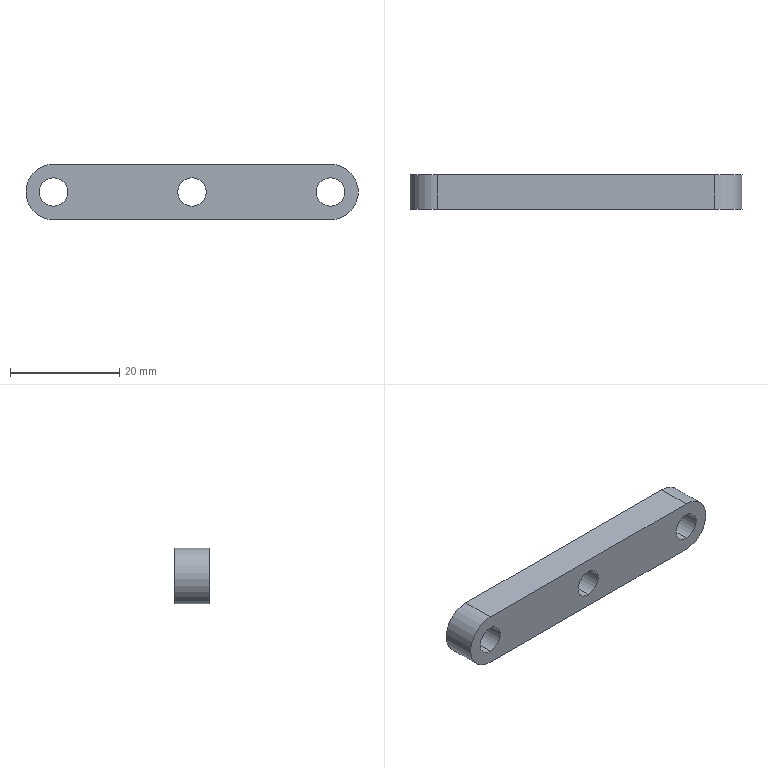Part | SolidWorks | features ICE 2, Extrusion 1 | 1 solid | 12 faces | box 60.96 x 6.35 x 10.16 mm | volume 3387 mm3 | cylinder 8 | plane 4 | commonest cylinder face diameters 5.207 x6 10.16 x2
STEP:
#1=CARTESIAN_POINT('',(25.4,0.,-2.604));
#2=VERTEX_POINT('',#1);
#3=CARTESIAN_POINT('',(25.4,0.,2.604));
#4=VERTEX_POINT('',#3);
#5=CARTESIAN_POINT('',(25.4,0.,0.));
#6=DIRECTION('',(0.,1.,0.));
#7=DIRECTION('',(0.,0.,1.));
#8=AXIS2_PLACEMENT_3D('',#5,#6,#7);
#9=CIRCLE('',#8,2.604);
#10=EDGE_CURVE('',#2,#4,#9,.T.);
#11=ORIENTED_EDGE('',*,*,#10,.F.);
#12=CARTESIAN_POINT('',(25.4,6.35,-2.604));
#13=VERTEX_POINT('',#12);
#14=CARTESIAN_POINT('',(25.4,0.,-2.604));
#15=DIRECTION('',(0.,1.,0.));
#16=VECTOR('',#15,1000.);
#17=LINE('',#14,#16);
#18=EDGE_CURVE('',#2,#13,#17,.T.);
#19=ORIENTED_EDGE('',*,*,#18,.T.);
#20=CARTESIAN_POINT('',(25.4,6.35,2.604));
#21=VERTEX_POINT('',#20);
#22=CARTESIAN_POINT('',(25.4,6.35,0.));
#23=DIRECTION('',(0.,1.,0.));
#24=DIRECTION('',(0.,0.,1.));
#25=AXIS2_PLACEMENT_3D('',#22,#23,#24);
#26=CIRCLE('',#25,2.604);
#27=EDGE_CURVE('',#13,#21,#26,.T.);
#28=ORIENTED_EDGE('',*,*,#27,.T.);
#29=CARTESIAN_POINT('',(25.4,0.,2.604));
#30=DIRECTION('',(0.,1.,0.));
#31=VECTOR('',#30,1000.);
#32=LINE('',#29,#31);
#33=EDGE_CURVE('',#4,#21,#32,.T.);
#34=ORIENTED_EDGE('',*,*,#33,.F.);
#35=EDGE_LOOP('',(#11,#19,#28,#34));
#36=FACE_OUTER_BOUND('',#35,.T.);
#37=CARTESIAN_POINT('',(25.4,0.,0.));
#38=DIRECTION('',(0.,1.,0.));
#39=DIRECTION('',(0.,0.,1.));
#40=AXIS2_PLACEMENT_3D('',#37,#38,#39);
#41=CYLINDRICAL_SURFACE('',#40,2.604);
#42=ADVANCED_FACE('',(#36),#41,.F.);
#43=CARTESIAN_POINT('',(50.8,0.,-2.604));
#44=VERTEX_POINT('',#43);
#45=CARTESIAN_POINT('',(50.8,0.,2.604));
#46=VERTEX_POINT('',#45);
#47=CARTESIAN_POINT('',(50.8,0.,0.));
#48=DIRECTION('',(0.,1.,0.));
#49=DIRECTION('',(0.,0.,-1.));
#50=AXIS2_PLACEMENT_3D('',#47,#48,#49);
#51=CIRCLE('',#50,2.604);
#52=EDGE_CURVE('',#44,#46,#51,.T.);
#53=ORIENTED_EDGE('',*,*,#52,.F.);
#54=CARTESIAN_POINT('',(50.8,6.35,-2.604));
#55=VERTEX_POINT('',#54);
#56=CARTESIAN_POINT('',(50.8,-8.202,-2.604));
#57=DIRECTION('',(0.,1.,0.));
#58=VECTOR('',#57,1000.);
#59=LINE('',#56,#58);
#60=EDGE_CURVE('',#44,#55,#59,.T.);
#61=ORIENTED_EDGE('',*,*,#60,.T.);
#62=CARTESIAN_POINT('',(50.8,6.35,2.604));
#63=VERTEX_POINT('',#62);
#64=CARTESIAN_POINT('',(50.8,6.35,0.));
#65=DIRECTION('',(0.,1.,0.));
#66=DIRECTION('',(0.,0.,1.));
#67=AXIS2_PLACEMENT_3D('',#64,#65,#66);
#68=CIRCLE('',#67,2.604);
#69=EDGE_CURVE('',#55,#63,#68,.T.);
#70=ORIENTED_EDGE('',*,*,#69,.T.);
#71=CARTESIAN_POINT('',(50.8,-8.202,2.604));
#72=DIRECTION('',(0.,1.,0.));
#73=VECTOR('',#72,1000.);
#74=LINE('',#71,#73);
#75=EDGE_CURVE('',#46,#63,#74,.T.);
#76=ORIENTED_EDGE('',*,*,#75,.F.);
#77=EDGE_LOOP('',(#53,#61,#70,#76));
#78=FACE_OUTER_BOUND('',#77,.T.);
#79=CARTESIAN_POINT('',(50.8,-8.202,0.));
#80=DIRECTION('',(0.,1.,0.));
#81=DIRECTION('',(0.,0.,1.));
#82=AXIS2_PLACEMENT_3D('',#79,#80,#81);
#83=CYLINDRICAL_SURFACE('',#82,2.604);
#84=ADVANCED_FACE('',(#78),#83,.F.);
#85=CARTESIAN_POINT('',(0.,0.,-2.603));
#86=VERTEX_POINT('',#85);
#87=CARTESIAN_POINT('',(0.,0.,2.603));
#88=VERTEX_POINT('',#87);
#89=CARTESIAN_POINT('',(0.,0.,0.));
#90=DIRECTION('',(0.,1.,0.));
#91=DIRECTION('',(0.,0.,-1.));
#92=AXIS2_PLACEMENT_3D('',#89,#90,#91);
#93=CIRCLE('',#92,2.603);
#94=EDGE_CURVE('',#86,#88,#93,.T.);
#95=ORIENTED_EDGE('',*,*,#94,.F.);
#96=CARTESIAN_POINT('',(0.,6.35,-2.603));
#97=VERTEX_POINT('',#96);
#98=CARTESIAN_POINT('',(0.,-8.202,-2.603));
#99=DIRECTION('',(0.,1.,0.));
#100=VECTOR('',#99,1000.);
#101=LINE('',#98,#100);
#102=EDGE_CURVE('',#86,#97,#101,.T.);
#103=ORIENTED_EDGE('',*,*,#102,.T.);
#104=CARTESIAN_POINT('',(0.,6.35,2.603));
#105=VERTEX_POINT('',#104);
#106=CARTESIAN_POINT('',(0.,6.35,0.));
#107=DIRECTION('',(0.,1.,0.));
#108=DIRECTION('',(0.,0.,1.));
#109=AXIS2_PLACEMENT_3D('',#106,#107,#108);
#110=CIRCLE('',#109,2.603);
#111=EDGE_CURVE('',#97,#105,#110,.T.);
#112=ORIENTED_EDGE('',*,*,#111,.T.);
#113=CARTESIAN_POINT('',(0.,-8.202,2.603));
#114=DIRECTION('',(0.,1.,0.));
#115=VECTOR('',#114,1000.);
#116=LINE('',#113,#115);
#117=EDGE_CURVE('',#88,#105,#116,.T.);
#118=ORIENTED_EDGE('',*,*,#117,.F.);
#119=EDGE_LOOP('',(#95,#103,#112,#118));
#120=FACE_OUTER_BOUND('',#119,.T.);
#121=CARTESIAN_POINT('',(0.,-8.202,0.));
#122=DIRECTION('',(0.,1.,0.));
#123=DIRECTION('',(0.,0.,1.));
#124=AXIS2_PLACEMENT_3D('',#121,#122,#123);
#125=CYLINDRICAL_SURFACE('',#124,2.603);
#126=ADVANCED_FACE('',(#120),#125,.F.);
#127=CARTESIAN_POINT('',(25.4,6.35,0.));
#128=DIRECTION('',(0.,1.,0.));
#129=DIRECTION('',(0.,0.,1.));
#130=AXIS2_PLACEMENT_3D('',#127,#128,#129);
#131=CIRCLE('',#130,2.604);
#132=EDGE_CURVE('',#21,#13,#131,.T.);
#133=ORIENTED_EDGE('',*,*,#132,.F.);
#134=ORIENTED_EDGE('',*,*,#27,.F.);
#135=EDGE_LOOP('',(#133,#134));
#136=FACE_BOUND('',#135,.T.);
#137=CARTESIAN_POINT('',(0.,6.35,-5.08));
#138=VERTEX_POINT('',#137);
#139=CARTESIAN_POINT('',(0.,6.35,5.08));
#140=VERTEX_POINT('',#139);
#141=CARTESIAN_POINT('',(0.,6.35,0.));
#142=DIRECTION('',(0.,1.,0.));
#143=DIRECTION('',(0.,0.,-1.));
#144=AXIS2_PLACEMENT_3D('',#141,#142,#143);
#145=CIRCLE('',#144,5.08);
#146=EDGE_CURVE('',#138,#140,#145,.T.);
#147=ORIENTED_EDGE('',*,*,#146,.T.);
#148=CARTESIAN_POINT('',(50.8,6.35,5.08));
#149=VERTEX_POINT('',#148);
#150=CARTESIAN_POINT('',(0.,6.35,5.08));
#151=DIRECTION('',(1.,0.,0.));
#152=VECTOR('',#151,1000.);
#153=LINE('',#150,#152);
#154=EDGE_CURVE('',#140,#149,#153,.T.);
#155=ORIENTED_EDGE('',*,*,#154,.T.);
#156=CARTESIAN_POINT('',(50.8,6.35,-5.08));
#157=VERTEX_POINT('',#156);
#158=CARTESIAN_POINT('',(50.8,6.35,0.));
#159=DIRECTION('',(0.,1.,0.));
#160=DIRECTION('',(0.,0.,-1.));
#161=AXIS2_PLACEMENT_3D('',#158,#159,#160);
#162=CIRCLE('',#161,5.08);
#163=EDGE_CURVE('',#149,#157,#162,.T.);
#164=ORIENTED_EDGE('',*,*,#163,.T.);
#165=CARTESIAN_POINT('',(0.,6.35,-5.08));
#166=DIRECTION('',(-1.,0.,0.));
#167=VECTOR('',#166,1000.);
#168=LINE('',#165,#167);
#169=EDGE_CURVE('',#157,#138,#168,.T.);
#170=ORIENTED_EDGE('',*,*,#169,.T.);
#171=EDGE_LOOP('',(#147,#155,#164,#170));
#172=FACE_OUTER_BOUND('',#171,.T.);
#173=CARTESIAN_POINT('',(0.,6.35,0.));
#174=DIRECTION('',(0.,1.,0.));
#175=DIRECTION('',(0.,0.,1.));
#176=AXIS2_PLACEMENT_3D('',#173,#174,#175);
#177=CIRCLE('',#176,2.603);
#178=EDGE_CURVE('',#105,#97,#177,.T.);
#179=ORIENTED_EDGE('',*,*,#178,.F.);
#180=ORIENTED_EDGE('',*,*,#111,.F.);
#181=EDGE_LOOP('',(#179,#180));
#182=FACE_BOUND('',#181,.T.);
#183=CARTESIAN_POINT('',(50.8,6.35,0.));
#184=DIRECTION('',(0.,1.,0.));
#185=DIRECTION('',(0.,0.,1.));
#186=AXIS2_PLACEMENT_3D('',#183,#184,#185);
#187=CIRCLE('',#186,2.604);
#188=EDGE_CURVE('',#63,#55,#187,.T.);
#189=ORIENTED_EDGE('',*,*,#188,.F.);
#190=ORIENTED_EDGE('',*,*,#69,.F.);
#191=EDGE_LOOP('',(#189,#190));
#192=FACE_BOUND('',#191,.T.);
#193=CARTESIAN_POINT('',(0.,6.35,0.));
#194=DIRECTION('',(0.,-1.,0.));
#195=DIRECTION('',(0.,0.,-1.));
#196=AXIS2_PLACEMENT_3D('',#193,#194,#195);
#197=PLANE('',#196);
#198=ADVANCED_FACE('',(#136,#172,#182,#192),#197,.F.);
#199=CARTESIAN_POINT('',(25.4,0.,0.));
#200=DIRECTION('',(0.,1.,0.));
#201=DIRECTION('',(0.,0.,1.));
#202=AXIS2_PLACEMENT_3D('',#199,#200,#201);
#203=CIRCLE('',#202,2.604);
#204=EDGE_CURVE('',#4,#2,#203,.T.);
#205=ORIENTED_EDGE('',*,*,#204,.T.);
#206=ORIENTED_EDGE('',*,*,#10,.T.);
#207=EDGE_LOOP('',(#205,#206));
#208=FACE_BOUND('',#207,.T.);
#209=CARTESIAN_POINT('',(0.,0.,-5.08));
#210=VERTEX_POINT('',#209);
#211=CARTESIAN_POINT('',(0.,0.,5.08));
#212=VERTEX_POINT('',#211);
#213=CARTESIAN_POINT('',(0.,0.,0.));
#214=DIRECTION('',(0.,1.,0.));
#215=DIRECTION('',(0.,0.,-1.));
#216=AXIS2_PLACEMENT_3D('',#213,#214,#215);
#217=CIRCLE('',#216,5.08);
#218=EDGE_CURVE('',#210,#212,#217,.T.);
#219=ORIENTED_EDGE('',*,*,#218,.F.);
#220=CARTESIAN_POINT('',(50.8,0.,-5.08));
#221=VERTEX_POINT('',#220);
#222=CARTESIAN_POINT('',(0.,0.,-5.08));
#223=DIRECTION('',(-1.,0.,0.));
#224=VECTOR('',#223,1000.);
#225=LINE('',#222,#224);
#226=EDGE_CURVE('',#221,#210,#225,.T.);
#227=ORIENTED_EDGE('',*,*,#226,.F.);
#228=CARTESIAN_POINT('',(50.8,0.,5.08));
#229=VERTEX_POINT('',#228);
#230=CARTESIAN_POINT('',(50.8,0.,0.));
#231=DIRECTION('',(0.,1.,0.));
#232=DIRECTION('',(0.,0.,-1.));
#233=AXIS2_PLACEMENT_3D('',#230,#231,#232);
#234=CIRCLE('',#233,5.08);
#235=EDGE_CURVE('',#229,#221,#234,.T.);
#236=ORIENTED_EDGE('',*,*,#235,.F.);
#237=CARTESIAN_POINT('',(0.,0.,5.08));
#238=DIRECTION('',(1.,0.,0.));
#239=VECTOR('',#238,1000.);
#240=LINE('',#237,#239);
#241=EDGE_CURVE('',#212,#229,#240,.T.);
#242=ORIENTED_EDGE('',*,*,#241,.F.);
#243=EDGE_LOOP('',(#219,#227,#236,#242));
#244=FACE_OUTER_BOUND('',#243,.T.);
#245=CARTESIAN_POINT('',(0.,0.,0.));
#246=DIRECTION('',(0.,1.,0.));
#247=DIRECTION('',(0.,0.,-1.));
#248=AXIS2_PLACEMENT_3D('',#245,#246,#247);
#249=CIRCLE('',#248,2.603);
#250=EDGE_CURVE('',#88,#86,#249,.T.);
#251=ORIENTED_EDGE('',*,*,#250,.T.);
#252=ORIENTED_EDGE('',*,*,#94,.T.);
#253=EDGE_LOOP('',(#251,#252));
#254=FACE_BOUND('',#253,.T.);
#255=CARTESIAN_POINT('',(50.8,0.,0.));
#256=DIRECTION('',(0.,1.,0.));
#257=DIRECTION('',(0.,0.,-1.));
#258=AXIS2_PLACEMENT_3D('',#255,#256,#257);
#259=CIRCLE('',#258,2.604);
#260=EDGE_CURVE('',#46,#44,#259,.T.);
#261=ORIENTED_EDGE('',*,*,#260,.T.);
#262=ORIENTED_EDGE('',*,*,#52,.T.);
#263=EDGE_LOOP('',(#261,#262));
#264=FACE_BOUND('',#263,.T.);
#265=CARTESIAN_POINT('',(0.,0.,0.));
#266=DIRECTION('',(0.,-1.,0.));
#267=DIRECTION('',(0.,0.,-1.));
#268=AXIS2_PLACEMENT_3D('',#265,#266,#267);
#269=PLANE('',#268);
#270=ADVANCED_FACE('',(#208,#244,#254,#264),#269,.T.);
#271=ORIENTED_EDGE('',*,*,#218,.T.);
#272=CARTESIAN_POINT('',(0.,6.35,5.08));
#273=DIRECTION('',(0.,-1.,0.));
#274=VECTOR('',#273,1000.);
#275=LINE('',#272,#274);
#276=EDGE_CURVE('',#140,#212,#275,.T.);
#277=ORIENTED_EDGE('',*,*,#276,.F.);
#278=ORIENTED_EDGE('',*,*,#146,.F.);
#279=CARTESIAN_POINT('',(0.,6.35,-5.08));
#280=DIRECTION('',(0.,-1.,0.));
#281=VECTOR('',#280,1000.);
#282=LINE('',#279,#281);
#283=EDGE_CURVE('',#138,#210,#282,.T.);
#284=ORIENTED_EDGE('',*,*,#283,.T.);
#285=EDGE_LOOP('',(#271,#277,#278,#284));
#286=FACE_OUTER_BOUND('',#285,.T.);
#287=CARTESIAN_POINT('',(0.,6.35,0.));
#288=DIRECTION('',(0.,-1.,0.));
#289=DIRECTION('',(0.,0.,-1.));
#290=AXIS2_PLACEMENT_3D('',#287,#288,#289);
#291=CYLINDRICAL_SURFACE('',#290,5.08);
#292=ADVANCED_FACE('',(#286),#291,.T.);
#293=ORIENTED_EDGE('',*,*,#241,.T.);
#294=CARTESIAN_POINT('',(50.8,6.35,5.08));
#295=DIRECTION('',(0.,-1.,0.));
#296=VECTOR('',#295,1000.);
#297=LINE('',#294,#296);
#298=EDGE_CURVE('',#149,#229,#297,.T.);
#299=ORIENTED_EDGE('',*,*,#298,.F.);
#300=ORIENTED_EDGE('',*,*,#154,.F.);
#301=ORIENTED_EDGE('',*,*,#276,.T.);
#302=EDGE_LOOP('',(#293,#299,#300,#301));
#303=FACE_OUTER_BOUND('',#302,.T.);
#304=CARTESIAN_POINT('',(0.,6.35,5.08));
#305=DIRECTION('',(0.,0.,-1.));
#306=DIRECTION('',(-1.,0.,0.));
#307=AXIS2_PLACEMENT_3D('',#304,#305,#306);
#308=PLANE('',#307);
#309=ADVANCED_FACE('',(#303),#308,.F.);
#310=ORIENTED_EDGE('',*,*,#235,.T.);
#311=CARTESIAN_POINT('',(50.8,6.35,-5.08));
#312=DIRECTION('',(0.,-1.,0.));
#313=VECTOR('',#312,1000.);
#314=LINE('',#311,#313);
#315=EDGE_CURVE('',#157,#221,#314,.T.);
#316=ORIENTED_EDGE('',*,*,#315,.F.);
#317=ORIENTED_EDGE('',*,*,#163,.F.);
#318=ORIENTED_EDGE('',*,*,#298,.T.);
#319=EDGE_LOOP('',(#310,#316,#317,#318));
#320=FACE_OUTER_BOUND('',#319,.T.);
#321=CARTESIAN_POINT('',(50.8,6.35,0.));
#322=DIRECTION('',(0.,-1.,0.));
#323=DIRECTION('',(0.,0.,-1.));
#324=AXIS2_PLACEMENT_3D('',#321,#322,#323);
#325=CYLINDRICAL_SURFACE('',#324,5.08);
#326=ADVANCED_FACE('',(#320),#325,.T.);
#327=ORIENTED_EDGE('',*,*,#226,.T.);
#328=ORIENTED_EDGE('',*,*,#283,.F.);
#329=ORIENTED_EDGE('',*,*,#169,.F.);
#330=ORIENTED_EDGE('',*,*,#315,.T.);
#331=EDGE_LOOP('',(#327,#328,#329,#330));
#332=FACE_OUTER_BOUND('',#331,.T.);
#333=CARTESIAN_POINT('',(0.,6.35,-5.08));
#334=DIRECTION('',(0.,0.,1.));
#335=DIRECTION('',(1.,0.,0.));
#336=AXIS2_PLACEMENT_3D('',#333,#334,#335);
#337=PLANE('',#336);
#338=ADVANCED_FACE('',(#332),#337,.F.);
#339=ORIENTED_EDGE('',*,*,#102,.F.);
#340=ORIENTED_EDGE('',*,*,#250,.F.);
#341=ORIENTED_EDGE('',*,*,#117,.T.);
#342=ORIENTED_EDGE('',*,*,#178,.T.);
#343=EDGE_LOOP('',(#339,#340,#341,#342));
#344=FACE_OUTER_BOUND('',#343,.T.);
#345=CARTESIAN_POINT('',(0.,-8.202,0.));
#346=DIRECTION('',(0.,1.,0.));
#347=DIRECTION('',(0.,0.,1.));
#348=AXIS2_PLACEMENT_3D('',#345,#346,#347);
#349=CYLINDRICAL_SURFACE('',#348,2.603);
#350=ADVANCED_FACE('',(#344),#349,.F.);
#351=ORIENTED_EDGE('',*,*,#60,.F.);
#352=ORIENTED_EDGE('',*,*,#260,.F.);
#353=ORIENTED_EDGE('',*,*,#75,.T.);
#354=ORIENTED_EDGE('',*,*,#188,.T.);
#355=EDGE_LOOP('',(#351,#352,#353,#354));
#356=FACE_OUTER_BOUND('',#355,.T.);
#357=CARTESIAN_POINT('',(50.8,-8.202,0.));
#358=DIRECTION('',(0.,1.,0.));
#359=DIRECTION('',(0.,0.,1.));
#360=AXIS2_PLACEMENT_3D('',#357,#358,#359);
#361=CYLINDRICAL_SURFACE('',#360,2.604);
#362=ADVANCED_FACE('',(#356),#361,.F.);
#363=ORIENTED_EDGE('',*,*,#18,.F.);
#364=ORIENTED_EDGE('',*,*,#204,.F.);
#365=ORIENTED_EDGE('',*,*,#33,.T.);
#366=ORIENTED_EDGE('',*,*,#132,.T.);
#367=EDGE_LOOP('',(#363,#364,#365,#366));
#368=FACE_OUTER_BOUND('',#367,.T.);
#369=CARTESIAN_POINT('',(25.4,0.,0.));
#370=DIRECTION('',(0.,1.,0.));
#371=DIRECTION('',(0.,0.,1.));
#372=AXIS2_PLACEMENT_3D('',#369,#370,#371);
#373=CYLINDRICAL_SURFACE('',#372,2.604);
#374=ADVANCED_FACE('',(#368),#373,.F.);
#375=CLOSED_SHELL('',(#42,#84,#126,#198,#270,#292,#309,#326,#338,#350,#362,#374));
#376=MANIFOLD_SOLID_BREP('',#375);
#377=CARTESIAN_POINT('',(0.,0.,0.));
#378=DIRECTION('',(0.,0.,1.));
#379=DIRECTION('',(1.,0.,0.));
#380=AXIS2_PLACEMENT_3D('',#377,#378,#379);
#381=(LENGTH_UNIT()NAMED_UNIT(*)SI_UNIT(.MILLI.,.METRE.));
#382=UNCERTAINTY_MEASURE_WITH_UNIT(LENGTH_MEASURE(0.00001),#381,'','');
#383=(NAMED_UNIT(*)PLANE_ANGLE_UNIT()SI_UNIT($,.RADIAN.));
#384=(NAMED_UNIT(*)SI_UNIT($,.STERADIAN.)SOLID_ANGLE_UNIT());
#385=(GEOMETRIC_REPRESENTATION_CONTEXT(3)GLOBAL_UNCERTAINTY_ASSIGNED_CONTEXT((#382))GLOBAL_UNIT_ASSIGNED_CONTEXT((#381,#383,#384))REPRESENTATION_CONTEXT('',''));
#386=ADVANCED_BREP_SHAPE_REPRESENTATION('',(#376,#380),#385);